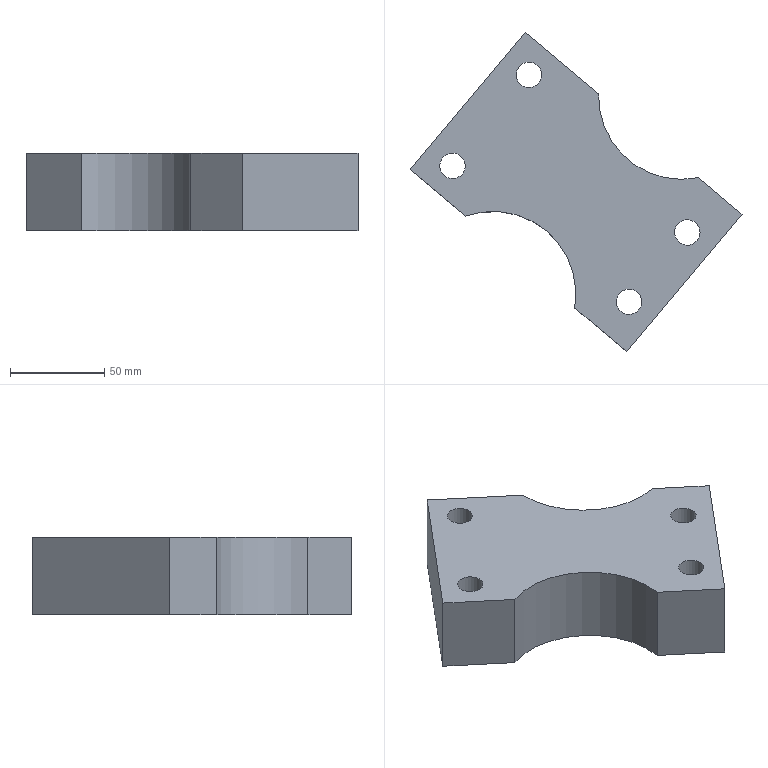Part | NX | features solid 2 | 1 solid | 22 faces | box 175.971 x 169.192 x 41 mm | volume 470118 mm3 | plane 12 | cylinder 10 | commonest cylinder face diameters 13.5 x4 20 x4 88 x2
STEP:
#1=CARTESIAN_POINT('',(1699.722,144.426,60.));
#2=VERTEX_POINT('',#1);
#3=CARTESIAN_POINT('',(1692.061,150.854,60.));
#4=DIRECTION('',(0.,0.,1.));
#5=DIRECTION('',(0.766,-0.6428,0.));
#6=AXIS2_PLACEMENT_3D('',#3,#4,#5);
#7=CIRCLE('',#6,10.);
#8=EDGE_CURVE('',#2,#2,#7,.T.);
#9=ORIENTED_EDGE('',*,*,#8,.T.);
#10=EDGE_LOOP('',(#9));
#11=FACE_BOUND('',#10,.T.);
#12=CARTESIAN_POINT('',(1575.261,179.675,60.));
#13=VERTEX_POINT('',#12);
#14=CARTESIAN_POINT('',(1567.6,186.102,60.));
#15=DIRECTION('',(0.,0.,1.));
#16=DIRECTION('',(0.766,-0.6428,0.));
#17=AXIS2_PLACEMENT_3D('',#14,#15,#16);
#18=CIRCLE('',#17,10.);
#19=EDGE_CURVE('',#13,#13,#18,.T.);
#20=ORIENTED_EDGE('',*,*,#19,.T.);
#21=EDGE_LOOP('',(#20));
#22=FACE_BOUND('',#21,.T.);
#23=CARTESIAN_POINT('',(1615.756,227.935,60.));
#24=VERTEX_POINT('',#23);
#25=CARTESIAN_POINT('',(1608.096,234.363,60.));
#26=DIRECTION('',(0.,0.,1.));
#27=DIRECTION('',(0.766,-0.6428,0.));
#28=AXIS2_PLACEMENT_3D('',#25,#26,#27);
#29=CIRCLE('',#28,10.);
#30=EDGE_CURVE('',#24,#24,#29,.T.);
#31=ORIENTED_EDGE('',*,*,#30,.T.);
#32=EDGE_LOOP('',(#31));
#33=FACE_BOUND('',#32,.T.);
#34=CARTESIAN_POINT('',(1668.868,107.656,60.));
#35=VERTEX_POINT('',#34);
#36=CARTESIAN_POINT('',(1661.208,114.084,60.));
#37=DIRECTION('',(0.,0.,1.));
#38=DIRECTION('',(0.766,-0.6428,0.));
#39=AXIS2_PLACEMENT_3D('',#36,#37,#38);
#40=CIRCLE('',#39,10.);
#41=EDGE_CURVE('',#35,#35,#40,.T.);
#42=ORIENTED_EDGE('',*,*,#41,.T.);
#43=EDGE_LOOP('',(#42));
#44=FACE_BOUND('',#43,.T.);
#45=CARTESIAN_POINT('',(1632.412,110.832,60.));
#46=VERTEX_POINT('',#45);
#47=CARTESIAN_POINT('',(1659.966,87.712,60.));
#48=VERTEX_POINT('',#47);
#49=CARTESIAN_POINT('',(1602.512,135.921,60.));
#50=DIRECTION('',(0.766,-0.6428,0.));
#51=VECTOR('',#50,1000.);
#52=LINE('',#49,#51);
#53=EDGE_CURVE('',#46,#48,#52,.T.);
#54=ORIENTED_EDGE('',*,*,#53,.F.);
#55=CARTESIAN_POINT('',(1574.403,159.508,60.));
#56=VERTEX_POINT('',#55);
#57=CARTESIAN_POINT('',(1589.,118.,60.));
#58=DIRECTION('',(0.,0.,1.));
#59=DIRECTION('',(-1.,0.,0.));
#60=AXIS2_PLACEMENT_3D('',#57,#58,#59);
#61=CIRCLE('',#60,44.);
#62=EDGE_CURVE('',#46,#56,#61,.T.);
#63=ORIENTED_EDGE('',*,*,#62,.T.);
#64=CARTESIAN_POINT('',(1545.059,184.13,60.));
#65=VERTEX_POINT('',#64);
#66=CARTESIAN_POINT('',(1602.512,135.921,60.));
#67=DIRECTION('',(0.766,-0.6428,0.));
#68=VECTOR('',#67,1000.);
#69=LINE('',#66,#68);
#70=EDGE_CURVE('',#65,#56,#69,.T.);
#71=ORIENTED_EDGE('',*,*,#70,.F.);
#72=CARTESIAN_POINT('',(1606.124,256.905,60.));
#73=VERTEX_POINT('',#72);
#74=CARTESIAN_POINT('',(1575.591,220.517,60.));
#75=DIRECTION('',(-0.6428,-0.766,0.));
#76=VECTOR('',#75,1000.);
#77=LINE('',#74,#76);
#78=EDGE_CURVE('',#73,#65,#77,.T.);
#79=ORIENTED_EDGE('',*,*,#78,.F.);
#80=CARTESIAN_POINT('',(1645.018,224.268,60.));
#81=VERTEX_POINT('',#80);
#82=CARTESIAN_POINT('',(1663.577,208.695,60.));
#83=DIRECTION('',(-0.766,0.6428,0.));
#84=VECTOR('',#83,1000.);
#85=LINE('',#82,#84);
#86=EDGE_CURVE('',#81,#73,#85,.T.);
#87=ORIENTED_EDGE('',*,*,#86,.F.);
#88=CARTESIAN_POINT('',(1697.886,179.907,60.));
#89=VERTEX_POINT('',#88);
#90=CARTESIAN_POINT('',(1689.,223.,60.));
#91=DIRECTION('',(0.,0.,1.));
#92=DIRECTION('',(-1.,0.,0.));
#93=AXIS2_PLACEMENT_3D('',#90,#91,#92);
#94=CIRCLE('',#93,44.);
#95=EDGE_CURVE('',#81,#89,#94,.T.);
#96=ORIENTED_EDGE('',*,*,#95,.T.);
#97=CARTESIAN_POINT('',(1721.031,160.486,60.));
#98=VERTEX_POINT('',#97);
#99=CARTESIAN_POINT('',(1663.577,208.695,60.));
#100=DIRECTION('',(-0.766,0.6428,0.));
#101=VECTOR('',#100,1000.);
#102=LINE('',#99,#101);
#103=EDGE_CURVE('',#98,#89,#102,.T.);
#104=ORIENTED_EDGE('',*,*,#103,.F.);
#105=CARTESIAN_POINT('',(1690.498,124.099,60.));
#106=DIRECTION('',(0.6428,0.766,0.));
#107=VECTOR('',#106,1000.);
#108=LINE('',#105,#107);
#109=EDGE_CURVE('',#48,#98,#108,.T.);
#110=ORIENTED_EDGE('',*,*,#109,.F.);
#111=EDGE_LOOP('',(#54,#63,#71,#79,#87,#96,#104,#110));
#112=FACE_BOUND('',#111,.T.);
#113=CARTESIAN_POINT('',(1633.045,172.308,60.));
#114=DIRECTION('',(0.,0.,-1.));
#115=DIRECTION('',(0.766,-0.6428,0.));
#116=AXIS2_PLACEMENT_3D('',#113,#114,#115);
#117=PLANE('',#116);
#118=ADVANCED_FACE('',(#11,#22,#33,#44,#112),#117,.T.);
#119=CARTESIAN_POINT('',(1613.267,230.024,101.));
#120=VERTEX_POINT('',#119);
#121=CARTESIAN_POINT('',(1608.096,234.363,101.));
#122=DIRECTION('',(0.,0.,1.));
#123=DIRECTION('',(0.766,-0.6428,0.));
#124=AXIS2_PLACEMENT_3D('',#121,#122,#123);
#125=CIRCLE('',#124,6.75);
#126=EDGE_CURVE('',#120,#120,#125,.T.);
#127=ORIENTED_EDGE('',*,*,#126,.F.);
#128=EDGE_LOOP('',(#127));
#129=FACE_BOUND('',#128,.T.);
#130=CARTESIAN_POINT('',(1572.771,181.764,101.));
#131=VERTEX_POINT('',#130);
#132=CARTESIAN_POINT('',(1567.6,186.102,101.));
#133=DIRECTION('',(0.,0.,1.));
#134=DIRECTION('',(0.766,-0.6428,0.));
#135=AXIS2_PLACEMENT_3D('',#132,#133,#134);
#136=CIRCLE('',#135,6.75);
#137=EDGE_CURVE('',#131,#131,#136,.T.);
#138=ORIENTED_EDGE('',*,*,#137,.F.);
#139=EDGE_LOOP('',(#138));
#140=FACE_BOUND('',#139,.T.);
#141=CARTESIAN_POINT('',(1666.378,109.745,101.));
#142=VERTEX_POINT('',#141);
#143=CARTESIAN_POINT('',(1661.208,114.084,101.));
#144=DIRECTION('',(0.,0.,1.));
#145=DIRECTION('',(0.766,-0.6428,0.));
#146=AXIS2_PLACEMENT_3D('',#143,#144,#145);
#147=CIRCLE('',#146,6.75);
#148=EDGE_CURVE('',#142,#142,#147,.T.);
#149=ORIENTED_EDGE('',*,*,#148,.F.);
#150=EDGE_LOOP('',(#149));
#151=FACE_BOUND('',#150,.T.);
#152=CARTESIAN_POINT('',(1697.232,146.515,101.));
#153=VERTEX_POINT('',#152);
#154=CARTESIAN_POINT('',(1692.061,150.854,101.));
#155=DIRECTION('',(0.,0.,1.));
#156=DIRECTION('',(0.766,-0.6428,0.));
#157=AXIS2_PLACEMENT_3D('',#154,#155,#156);
#158=CIRCLE('',#157,6.75);
#159=EDGE_CURVE('',#153,#153,#158,.T.);
#160=ORIENTED_EDGE('',*,*,#159,.F.);
#161=EDGE_LOOP('',(#160));
#162=FACE_BOUND('',#161,.T.);
#163=CARTESIAN_POINT('',(1574.403,159.508,101.));
#164=VERTEX_POINT('',#163);
#165=CARTESIAN_POINT('',(1545.059,184.13,101.));
#166=VERTEX_POINT('',#165);
#167=CARTESIAN_POINT('',(1602.512,135.921,101.));
#168=DIRECTION('',(-0.766,0.6428,0.));
#169=VECTOR('',#168,1000.);
#170=LINE('',#167,#169);
#171=EDGE_CURVE('',#164,#166,#170,.T.);
#172=ORIENTED_EDGE('',*,*,#171,.F.);
#173=CARTESIAN_POINT('',(1632.412,110.832,101.));
#174=VERTEX_POINT('',#173);
#175=CARTESIAN_POINT('',(1589.,118.,101.));
#176=DIRECTION('',(0.,0.,1.));
#177=DIRECTION('',(1.,0.,0.));
#178=AXIS2_PLACEMENT_3D('',#175,#176,#177);
#179=CIRCLE('',#178,44.);
#180=EDGE_CURVE('',#174,#164,#179,.T.);
#181=ORIENTED_EDGE('',*,*,#180,.F.);
#182=CARTESIAN_POINT('',(1659.966,87.712,101.));
#183=VERTEX_POINT('',#182);
#184=CARTESIAN_POINT('',(1602.512,135.921,101.));
#185=DIRECTION('',(-0.766,0.6428,0.));
#186=VECTOR('',#185,1000.);
#187=LINE('',#184,#186);
#188=EDGE_CURVE('',#183,#174,#187,.T.);
#189=ORIENTED_EDGE('',*,*,#188,.F.);
#190=CARTESIAN_POINT('',(1721.031,160.486,101.));
#191=VERTEX_POINT('',#190);
#192=CARTESIAN_POINT('',(1690.498,124.099,101.));
#193=DIRECTION('',(-0.6428,-0.766,0.));
#194=VECTOR('',#193,1000.);
#195=LINE('',#192,#194);
#196=EDGE_CURVE('',#191,#183,#195,.T.);
#197=ORIENTED_EDGE('',*,*,#196,.F.);
#198=CARTESIAN_POINT('',(1697.886,179.907,101.));
#199=VERTEX_POINT('',#198);
#200=CARTESIAN_POINT('',(1663.577,208.695,101.));
#201=DIRECTION('',(0.766,-0.6428,0.));
#202=VECTOR('',#201,1000.);
#203=LINE('',#200,#202);
#204=EDGE_CURVE('',#199,#191,#203,.T.);
#205=ORIENTED_EDGE('',*,*,#204,.F.);
#206=CARTESIAN_POINT('',(1645.018,224.268,101.));
#207=VERTEX_POINT('',#206);
#208=CARTESIAN_POINT('',(1689.,223.,101.));
#209=DIRECTION('',(0.,0.,1.));
#210=DIRECTION('',(1.,0.,0.));
#211=AXIS2_PLACEMENT_3D('',#208,#209,#210);
#212=CIRCLE('',#211,44.);
#213=EDGE_CURVE('',#207,#199,#212,.T.);
#214=ORIENTED_EDGE('',*,*,#213,.F.);
#215=CARTESIAN_POINT('',(1606.124,256.905,101.));
#216=VERTEX_POINT('',#215);
#217=CARTESIAN_POINT('',(1663.577,208.695,101.));
#218=DIRECTION('',(0.766,-0.6428,0.));
#219=VECTOR('',#218,1000.);
#220=LINE('',#217,#219);
#221=EDGE_CURVE('',#216,#207,#220,.T.);
#222=ORIENTED_EDGE('',*,*,#221,.F.);
#223=CARTESIAN_POINT('',(1575.591,220.517,101.));
#224=DIRECTION('',(0.6428,0.766,0.));
#225=VECTOR('',#224,1000.);
#226=LINE('',#223,#225);
#227=EDGE_CURVE('',#166,#216,#226,.T.);
#228=ORIENTED_EDGE('',*,*,#227,.F.);
#229=EDGE_LOOP('',(#172,#181,#189,#197,#205,#214,#222,#228));
#230=FACE_BOUND('',#229,.T.);
#231=CARTESIAN_POINT('',(1633.045,172.308,101.));
#232=DIRECTION('',(0.,0.,1.));
#233=DIRECTION('',(-0.766,0.6428,0.));
#234=AXIS2_PLACEMENT_3D('',#231,#232,#233);
#235=PLANE('',#234);
#236=ADVANCED_FACE('',(#129,#140,#151,#162,#230),#235,.T.);
#237=ORIENTED_EDGE('',*,*,#188,.T.);
#238=CARTESIAN_POINT('',(1632.412,110.832,-98.5));
#239=DIRECTION('',(0.,0.,-1.));
#240=VECTOR('',#239,1000.);
#241=LINE('',#238,#240);
#242=EDGE_CURVE('',#174,#46,#241,.T.);
#243=ORIENTED_EDGE('',*,*,#242,.T.);
#244=ORIENTED_EDGE('',*,*,#53,.T.);
#245=CARTESIAN_POINT('',(1659.966,87.712,81.));
#246=DIRECTION('',(0.,0.,1.));
#247=VECTOR('',#246,1000.);
#248=LINE('',#245,#247);
#249=EDGE_CURVE('',#48,#183,#248,.T.);
#250=ORIENTED_EDGE('',*,*,#249,.T.);
#251=EDGE_LOOP('',(#237,#243,#244,#250));
#252=FACE_BOUND('',#251,.T.);
#253=CARTESIAN_POINT('',(1602.512,135.921,81.));
#254=DIRECTION('',(-0.6428,-0.766,0.));
#255=DIRECTION('',(0.,0.,1.));
#256=AXIS2_PLACEMENT_3D('',#253,#254,#255);
#257=PLANE('',#256);
#258=ADVANCED_FACE('',(#252),#257,.T.);
#259=ORIENTED_EDGE('',*,*,#70,.T.);
#260=CARTESIAN_POINT('',(1574.403,159.508,-98.5));
#261=DIRECTION('',(0.,0.,1.));
#262=VECTOR('',#261,1000.);
#263=LINE('',#260,#262);
#264=EDGE_CURVE('',#56,#164,#263,.T.);
#265=ORIENTED_EDGE('',*,*,#264,.T.);
#266=ORIENTED_EDGE('',*,*,#171,.T.);
#267=CARTESIAN_POINT('',(1545.059,184.13,81.));
#268=DIRECTION('',(0.,0.,1.));
#269=VECTOR('',#268,1000.);
#270=LINE('',#267,#269);
#271=EDGE_CURVE('',#65,#166,#270,.T.);
#272=ORIENTED_EDGE('',*,*,#271,.F.);
#273=EDGE_LOOP('',(#259,#265,#266,#272));
#274=FACE_BOUND('',#273,.T.);
#275=CARTESIAN_POINT('',(1602.512,135.921,81.));
#276=DIRECTION('',(-0.6428,-0.766,0.));
#277=DIRECTION('',(0.,0.,1.));
#278=AXIS2_PLACEMENT_3D('',#275,#276,#277);
#279=PLANE('',#278);
#280=ADVANCED_FACE('',(#274),#279,.T.);
#281=CARTESIAN_POINT('',(1645.018,224.268,-98.5));
#282=DIRECTION('',(0.,0.,1.));
#283=VECTOR('',#282,1000.);
#284=LINE('',#281,#283);
#285=EDGE_CURVE('',#81,#207,#284,.T.);
#286=ORIENTED_EDGE('',*,*,#285,.F.);
#287=ORIENTED_EDGE('',*,*,#86,.T.);
#288=CARTESIAN_POINT('',(1606.124,256.905,81.));
#289=DIRECTION('',(0.,0.,1.));
#290=VECTOR('',#289,1000.);
#291=LINE('',#288,#290);
#292=EDGE_CURVE('',#73,#216,#291,.T.);
#293=ORIENTED_EDGE('',*,*,#292,.T.);
#294=ORIENTED_EDGE('',*,*,#221,.T.);
#295=EDGE_LOOP('',(#286,#287,#293,#294));
#296=FACE_BOUND('',#295,.T.);
#297=CARTESIAN_POINT('',(1663.577,208.695,81.));
#298=DIRECTION('',(0.6428,0.766,0.));
#299=DIRECTION('',(0.,0.,-1.));
#300=AXIS2_PLACEMENT_3D('',#297,#298,#299);
#301=PLANE('',#300);
#302=ADVANCED_FACE('',(#296),#301,.T.);
#303=ORIENTED_EDGE('',*,*,#271,.T.);
#304=ORIENTED_EDGE('',*,*,#227,.T.);
#305=ORIENTED_EDGE('',*,*,#292,.F.);
#306=ORIENTED_EDGE('',*,*,#78,.T.);
#307=EDGE_LOOP('',(#303,#304,#305,#306));
#308=FACE_BOUND('',#307,.T.);
#309=CARTESIAN_POINT('',(1575.591,220.517,81.));
#310=DIRECTION('',(-0.766,0.6428,0.));
#311=DIRECTION('',(0.,0.,-1.));
#312=AXIS2_PLACEMENT_3D('',#309,#310,#311);
#313=PLANE('',#312);
#314=ADVANCED_FACE('',(#308),#313,.T.);
#315=CARTESIAN_POINT('',(1697.886,179.907,-98.5));
#316=DIRECTION('',(0.,0.,-1.));
#317=VECTOR('',#316,1000.);
#318=LINE('',#315,#317);
#319=EDGE_CURVE('',#199,#89,#318,.T.);
#320=ORIENTED_EDGE('',*,*,#319,.F.);
#321=ORIENTED_EDGE('',*,*,#204,.T.);
#322=CARTESIAN_POINT('',(1721.031,160.486,81.));
#323=DIRECTION('',(0.,0.,1.));
#324=VECTOR('',#323,1000.);
#325=LINE('',#322,#324);
#326=EDGE_CURVE('',#98,#191,#325,.T.);
#327=ORIENTED_EDGE('',*,*,#326,.F.);
#328=ORIENTED_EDGE('',*,*,#103,.T.);
#329=EDGE_LOOP('',(#320,#321,#327,#328));
#330=FACE_BOUND('',#329,.T.);
#331=CARTESIAN_POINT('',(1663.577,208.695,81.));
#332=DIRECTION('',(0.6428,0.766,0.));
#333=DIRECTION('',(0.,0.,-1.));
#334=AXIS2_PLACEMENT_3D('',#331,#332,#333);
#335=PLANE('',#334);
#336=ADVANCED_FACE('',(#330),#335,.T.);
#337=ORIENTED_EDGE('',*,*,#109,.T.);
#338=ORIENTED_EDGE('',*,*,#326,.T.);
#339=ORIENTED_EDGE('',*,*,#196,.T.);
#340=ORIENTED_EDGE('',*,*,#249,.F.);
#341=EDGE_LOOP('',(#337,#338,#339,#340));
#342=FACE_BOUND('',#341,.T.);
#343=CARTESIAN_POINT('',(1690.498,124.099,81.));
#344=DIRECTION('',(0.766,-0.6428,0.));
#345=DIRECTION('',(0.,0.,1.));
#346=AXIS2_PLACEMENT_3D('',#343,#344,#345);
#347=PLANE('',#346);
#348=ADVANCED_FACE('',(#342),#347,.T.);
#349=ORIENTED_EDGE('',*,*,#126,.T.);
#350=EDGE_LOOP('',(#349));
#351=FACE_BOUND('',#350,.T.);
#352=CARTESIAN_POINT('',(1613.267,230.024,75.));
#353=VERTEX_POINT('',#352);
#354=CARTESIAN_POINT('',(1608.096,234.363,75.));
#355=DIRECTION('',(0.,0.,1.));
#356=DIRECTION('',(0.766,-0.6428,0.));
#357=AXIS2_PLACEMENT_3D('',#354,#355,#356);
#358=CIRCLE('',#357,6.75);
#359=EDGE_CURVE('',#353,#353,#358,.T.);
#360=ORIENTED_EDGE('',*,*,#359,.F.);
#361=EDGE_LOOP('',(#360));
#362=FACE_BOUND('',#361,.T.);
#363=CARTESIAN_POINT('',(1608.096,234.363,55.));
#364=DIRECTION('',(0.,0.,1.));
#365=DIRECTION('',(-0.766,0.6428,0.));
#366=AXIS2_PLACEMENT_3D('',#363,#364,#365);
#367=CYLINDRICAL_SURFACE('',#366,6.75);
#368=ADVANCED_FACE('',(#351,#362),#367,.F.);
#369=ORIENTED_EDGE('',*,*,#359,.T.);
#370=EDGE_LOOP('',(#369));
#371=FACE_BOUND('',#370,.T.);
#372=CARTESIAN_POINT('',(1615.756,227.935,75.));
#373=VERTEX_POINT('',#372);
#374=CARTESIAN_POINT('',(1608.096,234.363,75.));
#375=DIRECTION('',(0.,0.,1.));
#376=DIRECTION('',(0.766,-0.6428,0.));
#377=AXIS2_PLACEMENT_3D('',#374,#375,#376);
#378=CIRCLE('',#377,10.);
#379=EDGE_CURVE('',#373,#373,#378,.T.);
#380=ORIENTED_EDGE('',*,*,#379,.F.);
#381=EDGE_LOOP('',(#380));
#382=FACE_BOUND('',#381,.T.);
#383=CARTESIAN_POINT('',(1608.096,234.363,75.));
#384=DIRECTION('',(0.,0.,1.));
#385=DIRECTION('',(-0.766,0.6428,0.));
#386=AXIS2_PLACEMENT_3D('',#383,#384,#385);
#387=PLANE('',#386);
#388=ADVANCED_FACE('',(#371,#382),#387,.F.);
#389=ORIENTED_EDGE('',*,*,#379,.T.);
#390=EDGE_LOOP('',(#389));
#391=FACE_BOUND('',#390,.T.);
#392=ORIENTED_EDGE('',*,*,#30,.F.);
#393=EDGE_LOOP('',(#392));
#394=FACE_BOUND('',#393,.T.);
#395=CARTESIAN_POINT('',(1608.096,234.363,60.));
#396=DIRECTION('',(0.,0.,1.));
#397=DIRECTION('',(-0.766,0.6428,0.));
#398=AXIS2_PLACEMENT_3D('',#395,#396,#397);
#399=CYLINDRICAL_SURFACE('',#398,10.);
#400=ADVANCED_FACE('',(#391,#394),#399,.F.);
#401=ORIENTED_EDGE('',*,*,#137,.T.);
#402=EDGE_LOOP('',(#401));
#403=FACE_BOUND('',#402,.T.);
#404=CARTESIAN_POINT('',(1572.771,181.764,75.));
#405=VERTEX_POINT('',#404);
#406=CARTESIAN_POINT('',(1567.6,186.102,75.));
#407=DIRECTION('',(0.,0.,1.));
#408=DIRECTION('',(0.766,-0.6428,0.));
#409=AXIS2_PLACEMENT_3D('',#406,#407,#408);
#410=CIRCLE('',#409,6.75);
#411=EDGE_CURVE('',#405,#405,#410,.T.);
#412=ORIENTED_EDGE('',*,*,#411,.F.);
#413=EDGE_LOOP('',(#412));
#414=FACE_BOUND('',#413,.T.);
#415=CARTESIAN_POINT('',(1567.6,186.102,55.));
#416=DIRECTION('',(0.,0.,1.));
#417=DIRECTION('',(-0.766,0.6428,0.));
#418=AXIS2_PLACEMENT_3D('',#415,#416,#417);
#419=CYLINDRICAL_SURFACE('',#418,6.75);
#420=ADVANCED_FACE('',(#403,#414),#419,.F.);
#421=ORIENTED_EDGE('',*,*,#411,.T.);
#422=EDGE_LOOP('',(#421));
#423=FACE_BOUND('',#422,.T.);
#424=CARTESIAN_POINT('',(1575.261,179.675,75.));
#425=VERTEX_POINT('',#424);
#426=CARTESIAN_POINT('',(1567.6,186.102,75.));
#427=DIRECTION('',(0.,0.,1.));
#428=DIRECTION('',(0.766,-0.6428,0.));
#429=AXIS2_PLACEMENT_3D('',#426,#427,#428);
#430=CIRCLE('',#429,10.);
#431=EDGE_CURVE('',#425,#425,#430,.T.);
#432=ORIENTED_EDGE('',*,*,#431,.F.);
#433=EDGE_LOOP('',(#432));
#434=FACE_BOUND('',#433,.T.);
#435=CARTESIAN_POINT('',(1567.6,186.102,75.));
#436=DIRECTION('',(0.,0.,1.));
#437=DIRECTION('',(-0.766,0.6428,0.));
#438=AXIS2_PLACEMENT_3D('',#435,#436,#437);
#439=PLANE('',#438);
#440=ADVANCED_FACE('',(#423,#434),#439,.F.);
#441=ORIENTED_EDGE('',*,*,#431,.T.);
#442=EDGE_LOOP('',(#441));
#443=FACE_BOUND('',#442,.T.);
#444=ORIENTED_EDGE('',*,*,#19,.F.);
#445=EDGE_LOOP('',(#444));
#446=FACE_BOUND('',#445,.T.);
#447=CARTESIAN_POINT('',(1567.6,186.102,60.));
#448=DIRECTION('',(0.,0.,1.));
#449=DIRECTION('',(-0.766,0.6428,0.));
#450=AXIS2_PLACEMENT_3D('',#447,#448,#449);
#451=CYLINDRICAL_SURFACE('',#450,10.);
#452=ADVANCED_FACE('',(#443,#446),#451,.F.);
#453=ORIENTED_EDGE('',*,*,#148,.T.);
#454=EDGE_LOOP('',(#453));
#455=FACE_BOUND('',#454,.T.);
#456=CARTESIAN_POINT('',(1666.378,109.745,75.));
#457=VERTEX_POINT('',#456);
#458=CARTESIAN_POINT('',(1661.208,114.084,75.));
#459=DIRECTION('',(0.,0.,1.));
#460=DIRECTION('',(0.766,-0.6428,0.));
#461=AXIS2_PLACEMENT_3D('',#458,#459,#460);
#462=CIRCLE('',#461,6.75);
#463=EDGE_CURVE('',#457,#457,#462,.T.);
#464=ORIENTED_EDGE('',*,*,#463,.F.);
#465=EDGE_LOOP('',(#464));
#466=FACE_BOUND('',#465,.T.);
#467=CARTESIAN_POINT('',(1661.208,114.084,55.));
#468=DIRECTION('',(0.,0.,1.));
#469=DIRECTION('',(-0.766,0.6428,0.));
#470=AXIS2_PLACEMENT_3D('',#467,#468,#469);
#471=CYLINDRICAL_SURFACE('',#470,6.75);
#472=ADVANCED_FACE('',(#455,#466),#471,.F.);
#473=ORIENTED_EDGE('',*,*,#463,.T.);
#474=EDGE_LOOP('',(#473));
#475=FACE_BOUND('',#474,.T.);
#476=CARTESIAN_POINT('',(1668.868,107.656,75.));
#477=VERTEX_POINT('',#476);
#478=CARTESIAN_POINT('',(1661.208,114.084,75.));
#479=DIRECTION('',(0.,0.,1.));
#480=DIRECTION('',(0.766,-0.6428,0.));
#481=AXIS2_PLACEMENT_3D('',#478,#479,#480);
#482=CIRCLE('',#481,10.);
#483=EDGE_CURVE('',#477,#477,#482,.T.);
#484=ORIENTED_EDGE('',*,*,#483,.F.);
#485=EDGE_LOOP('',(#484));
#486=FACE_BOUND('',#485,.T.);
#487=CARTESIAN_POINT('',(1657.994,110.254,75.));
#488=DIRECTION('',(0.,0.,1.));
#489=DIRECTION('',(-0.766,0.6428,0.));
#490=AXIS2_PLACEMENT_3D('',#487,#488,#489);
#491=PLANE('',#490);
#492=ADVANCED_FACE('',(#475,#486),#491,.F.);
#493=ORIENTED_EDGE('',*,*,#483,.T.);
#494=EDGE_LOOP('',(#493));
#495=FACE_BOUND('',#494,.T.);
#496=ORIENTED_EDGE('',*,*,#41,.F.);
#497=EDGE_LOOP('',(#496));
#498=FACE_BOUND('',#497,.T.);
#499=CARTESIAN_POINT('',(1661.208,114.084,60.));
#500=DIRECTION('',(0.,0.,1.));
#501=DIRECTION('',(-0.766,0.6428,0.));
#502=AXIS2_PLACEMENT_3D('',#499,#500,#501);
#503=CYLINDRICAL_SURFACE('',#502,10.);
#504=ADVANCED_FACE('',(#495,#498),#503,.F.);
#505=ORIENTED_EDGE('',*,*,#159,.T.);
#506=EDGE_LOOP('',(#505));
#507=FACE_BOUND('',#506,.T.);
#508=CARTESIAN_POINT('',(1697.232,146.515,75.));
#509=VERTEX_POINT('',#508);
#510=CARTESIAN_POINT('',(1692.061,150.854,75.));
#511=DIRECTION('',(0.,0.,1.));
#512=DIRECTION('',(0.766,-0.6428,0.));
#513=AXIS2_PLACEMENT_3D('',#510,#511,#512);
#514=CIRCLE('',#513,6.75);
#515=EDGE_CURVE('',#509,#509,#514,.T.);
#516=ORIENTED_EDGE('',*,*,#515,.F.);
#517=EDGE_LOOP('',(#516));
#518=FACE_BOUND('',#517,.T.);
#519=CARTESIAN_POINT('',(1692.061,150.854,55.));
#520=DIRECTION('',(0.,0.,1.));
#521=DIRECTION('',(-0.766,0.6428,0.));
#522=AXIS2_PLACEMENT_3D('',#519,#520,#521);
#523=CYLINDRICAL_SURFACE('',#522,6.75);
#524=ADVANCED_FACE('',(#507,#518),#523,.F.);
#525=ORIENTED_EDGE('',*,*,#515,.T.);
#526=EDGE_LOOP('',(#525));
#527=FACE_BOUND('',#526,.T.);
#528=CARTESIAN_POINT('',(1699.722,144.426,75.));
#529=VERTEX_POINT('',#528);
#530=CARTESIAN_POINT('',(1692.061,150.854,75.));
#531=DIRECTION('',(0.,0.,1.));
#532=DIRECTION('',(0.766,-0.6428,0.));
#533=AXIS2_PLACEMENT_3D('',#530,#531,#532);
#534=CIRCLE('',#533,10.);
#535=EDGE_CURVE('',#529,#529,#534,.T.);
#536=ORIENTED_EDGE('',*,*,#535,.F.);
#537=EDGE_LOOP('',(#536));
#538=FACE_BOUND('',#537,.T.);
#539=CARTESIAN_POINT('',(1698.489,158.514,75.));
#540=DIRECTION('',(0.,0.,1.));
#541=DIRECTION('',(-0.766,0.6428,0.));
#542=AXIS2_PLACEMENT_3D('',#539,#540,#541);
#543=PLANE('',#542);
#544=ADVANCED_FACE('',(#527,#538),#543,.F.);
#545=ORIENTED_EDGE('',*,*,#535,.T.);
#546=EDGE_LOOP('',(#545));
#547=FACE_BOUND('',#546,.T.);
#548=ORIENTED_EDGE('',*,*,#8,.F.);
#549=EDGE_LOOP('',(#548));
#550=FACE_BOUND('',#549,.T.);
#551=CARTESIAN_POINT('',(1692.061,150.854,60.));
#552=DIRECTION('',(0.,0.,1.));
#553=DIRECTION('',(-0.766,0.6428,0.));
#554=AXIS2_PLACEMENT_3D('',#551,#552,#553);
#555=CYLINDRICAL_SURFACE('',#554,10.);
#556=ADVANCED_FACE('',(#547,#550),#555,.F.);
#557=ORIENTED_EDGE('',*,*,#285,.T.);
#558=ORIENTED_EDGE('',*,*,#213,.T.);
#559=ORIENTED_EDGE('',*,*,#319,.T.);
#560=ORIENTED_EDGE('',*,*,#95,.F.);
#561=EDGE_LOOP('',(#557,#558,#559,#560));
#562=FACE_BOUND('',#561,.T.);
#563=CARTESIAN_POINT('',(1689.,223.,-98.5));
#564=DIRECTION('',(0.,0.,1.));
#565=DIRECTION('',(-1.,0.,0.));
#566=AXIS2_PLACEMENT_3D('',#563,#564,#565);
#567=CYLINDRICAL_SURFACE('',#566,44.);
#568=ADVANCED_FACE('',(#562),#567,.F.);
#569=ORIENTED_EDGE('',*,*,#242,.F.);
#570=ORIENTED_EDGE('',*,*,#180,.T.);
#571=ORIENTED_EDGE('',*,*,#264,.F.);
#572=ORIENTED_EDGE('',*,*,#62,.F.);
#573=EDGE_LOOP('',(#569,#570,#571,#572));
#574=FACE_BOUND('',#573,.T.);
#575=CARTESIAN_POINT('',(1589.,118.,-98.5));
#576=DIRECTION('',(0.,0.,1.));
#577=DIRECTION('',(-1.,0.,0.));
#578=AXIS2_PLACEMENT_3D('',#575,#576,#577);
#579=CYLINDRICAL_SURFACE('',#578,44.);
#580=ADVANCED_FACE('',(#574),#579,.F.);
#581=CLOSED_SHELL('',(#118,#236,#258,#280,#302,#314,#336,#348,#368,#388,#400,#420,#440,#452,#472,#492,#504,#524,#544,#556,#568,#580));
#582=MANIFOLD_SOLID_BREP('',#581);
#583=(LENGTH_UNIT()NAMED_UNIT(*)SI_UNIT(.MILLI.,.METRE.));
#584=UNCERTAINTY_MEASURE_WITH_UNIT(LENGTH_MEASURE(0.00001),#583,'','');
#585=(NAMED_UNIT(*)PLANE_ANGLE_UNIT()SI_UNIT($,.RADIAN.));
#586=(NAMED_UNIT(*)SI_UNIT($,.STERADIAN.)SOLID_ANGLE_UNIT());
#587=(GEOMETRIC_REPRESENTATION_CONTEXT(3)GLOBAL_UNCERTAINTY_ASSIGNED_CONTEXT((#584))GLOBAL_UNIT_ASSIGNED_CONTEXT((#583,#585,#586))REPRESENTATION_CONTEXT('',''));
#588=ADVANCED_BREP_SHAPE_REPRESENTATION('',(#582),#587);